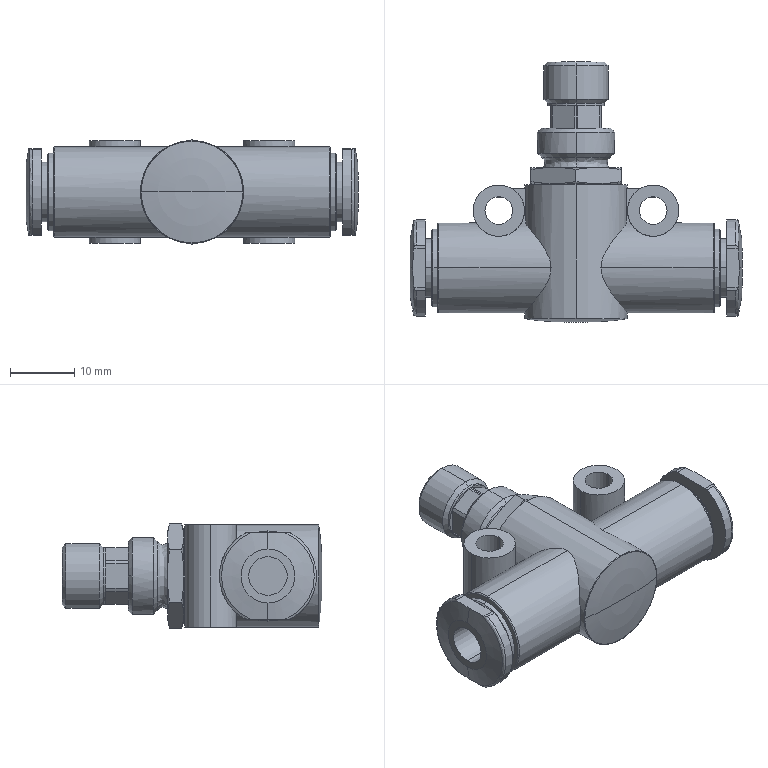Part | SolidWorks | features BaseBody 1 | 1 solid | 137 faces | box 51.6 x 40.42 x 16.166 mm | volume 11359 mm3 | cylinder 53 | plane 41 | cone 29 | spline 12 | torus 2 | commonest cylinder face diameters 6 x12 8.8 x7 14 x6 4.3 x4 8 x4 9.24 x4